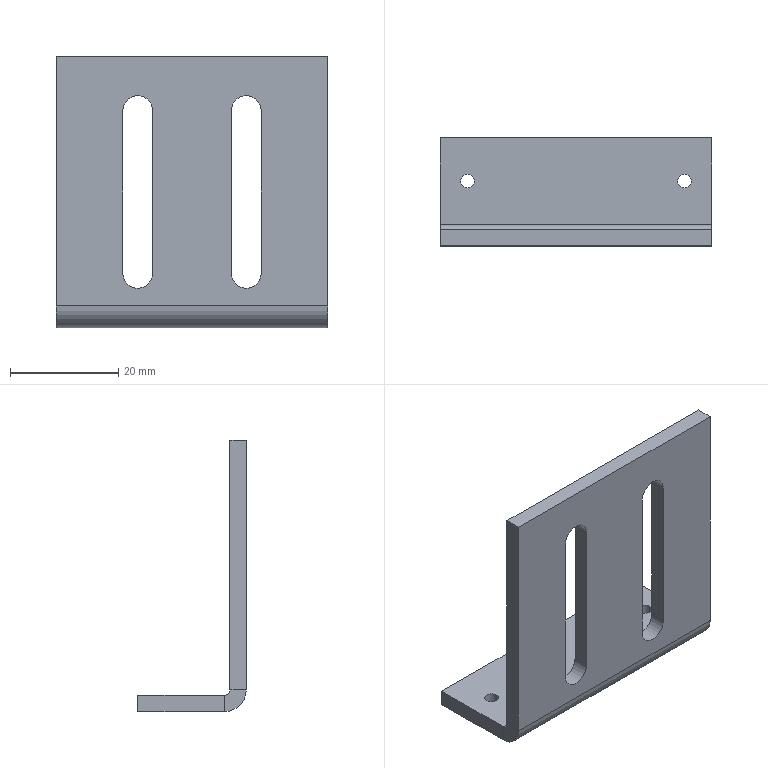Part | SolidWorks | features EdgeFlange 1, FlatPattern 1, HoleWzd 1, ICE 1, SMBaseFlange 1, SheetMetal 1 | 1 solid | 28 faces | box 50 x 20 x 50 mm | volume 8727 mm3 | plane 16 | cylinder 12 | commonest cylinder face diameters 5.5 x6 2.5 x4 2 x1 8 x1
STEP:
#1=CARTESIAN_POINT('',(18.75,2.,0.));
#2=VERTEX_POINT('',#1);
#3=CARTESIAN_POINT('',(21.25,2.,0.));
#4=VERTEX_POINT('',#3);
#5=CARTESIAN_POINT('',(20.,2.,0.));
#6=DIRECTION('',(0.,0.,1.));
#7=DIRECTION('',(1.,0.,0.));
#8=AXIS2_PLACEMENT_3D('',#5,#6,#7);
#9=CIRCLE('',#8,1.25);
#10=EDGE_CURVE('',#2,#4,#9,.T.);
#11=ORIENTED_EDGE('',*,*,#10,.T.);
#12=CARTESIAN_POINT('',(21.25,2.,-3.));
#13=VERTEX_POINT('',#12);
#14=CARTESIAN_POINT('',(21.25,2.,-3.));
#15=DIRECTION('',(0.,0.,-1.));
#16=VECTOR('',#15,1000.);
#17=LINE('',#14,#16);
#18=EDGE_CURVE('',#4,#13,#17,.T.);
#19=ORIENTED_EDGE('',*,*,#18,.T.);
#20=CARTESIAN_POINT('',(18.75,2.,-3.));
#21=VERTEX_POINT('',#20);
#22=CARTESIAN_POINT('',(20.,2.,-3.));
#23=DIRECTION('',(0.,0.,-1.));
#24=DIRECTION('',(-1.,0.,0.));
#25=AXIS2_PLACEMENT_3D('',#22,#23,#24);
#26=CIRCLE('',#25,1.25);
#27=EDGE_CURVE('',#13,#21,#26,.T.);
#28=ORIENTED_EDGE('',*,*,#27,.T.);
#29=CARTESIAN_POINT('',(18.75,2.,-3.));
#30=DIRECTION('',(0.,0.,-1.));
#31=VECTOR('',#30,1000.);
#32=LINE('',#29,#31);
#33=EDGE_CURVE('',#2,#21,#32,.T.);
#34=ORIENTED_EDGE('',*,*,#33,.F.);
#35=EDGE_LOOP('',(#11,#19,#28,#34));
#36=FACE_OUTER_BOUND('',#35,.T.);
#37=CARTESIAN_POINT('',(20.,2.,-3.));
#38=DIRECTION('',(0.,0.,-1.));
#39=DIRECTION('',(-1.,0.,0.));
#40=AXIS2_PLACEMENT_3D('',#37,#38,#39);
#41=CYLINDRICAL_SURFACE('',#40,1.25);
#42=ADVANCED_FACE('',(#36),#41,.F.);
#43=CARTESIAN_POINT('',(-21.25,2.,0.));
#44=VERTEX_POINT('',#43);
#45=CARTESIAN_POINT('',(-18.75,2.,0.));
#46=VERTEX_POINT('',#45);
#47=CARTESIAN_POINT('',(-20.,2.,0.));
#48=DIRECTION('',(0.,0.,1.));
#49=DIRECTION('',(1.,0.,0.));
#50=AXIS2_PLACEMENT_3D('',#47,#48,#49);
#51=CIRCLE('',#50,1.25);
#52=EDGE_CURVE('',#44,#46,#51,.T.);
#53=ORIENTED_EDGE('',*,*,#52,.T.);
#54=CARTESIAN_POINT('',(-18.75,2.,-3.));
#55=VERTEX_POINT('',#54);
#56=CARTESIAN_POINT('',(-18.75,2.,-3.));
#57=DIRECTION('',(0.,0.,-1.));
#58=VECTOR('',#57,1000.);
#59=LINE('',#56,#58);
#60=EDGE_CURVE('',#46,#55,#59,.T.);
#61=ORIENTED_EDGE('',*,*,#60,.T.);
#62=CARTESIAN_POINT('',(-21.25,2.,-3.));
#63=VERTEX_POINT('',#62);
#64=CARTESIAN_POINT('',(-20.,2.,-3.));
#65=DIRECTION('',(0.,0.,-1.));
#66=DIRECTION('',(-1.,0.,0.));
#67=AXIS2_PLACEMENT_3D('',#64,#65,#66);
#68=CIRCLE('',#67,1.25);
#69=EDGE_CURVE('',#55,#63,#68,.T.);
#70=ORIENTED_EDGE('',*,*,#69,.T.);
#71=CARTESIAN_POINT('',(-21.25,2.,-3.));
#72=DIRECTION('',(0.,0.,-1.));
#73=VECTOR('',#72,1000.);
#74=LINE('',#71,#73);
#75=EDGE_CURVE('',#44,#63,#74,.T.);
#76=ORIENTED_EDGE('',*,*,#75,.F.);
#77=EDGE_LOOP('',(#53,#61,#70,#76));
#78=FACE_OUTER_BOUND('',#77,.T.);
#79=CARTESIAN_POINT('',(-20.,2.,-3.));
#80=DIRECTION('',(0.,0.,-1.));
#81=DIRECTION('',(-1.,0.,0.));
#82=AXIS2_PLACEMENT_3D('',#79,#80,#81);
#83=CYLINDRICAL_SURFACE('',#82,1.25);
#84=ADVANCED_FACE('',(#78),#83,.F.);
#85=CARTESIAN_POINT('',(10.,-10.,39.75));
#86=VERTEX_POINT('',#85);
#87=CARTESIAN_POINT('',(12.75,-10.,37.));
#88=VERTEX_POINT('',#87);
#89=CARTESIAN_POINT('',(10.,-10.,37.));
#90=DIRECTION('',(0.,1.,0.));
#91=DIRECTION('',(0.,0.,1.));
#92=AXIS2_PLACEMENT_3D('',#89,#90,#91);
#93=CIRCLE('',#92,2.75);
#94=EDGE_CURVE('',#86,#88,#93,.T.);
#95=ORIENTED_EDGE('',*,*,#94,.F.);
#96=CARTESIAN_POINT('',(10.,-7.,39.75));
#97=VERTEX_POINT('',#96);
#98=CARTESIAN_POINT('',(10.,-17.,39.75));
#99=DIRECTION('',(0.,1.,0.));
#100=VECTOR('',#99,1000.);
#101=LINE('',#98,#100);
#102=EDGE_CURVE('',#86,#97,#101,.T.);
#103=ORIENTED_EDGE('',*,*,#102,.T.);
#104=CARTESIAN_POINT('',(12.75,-7.,37.));
#105=VERTEX_POINT('',#104);
#106=CARTESIAN_POINT('',(10.,-7.,37.));
#107=DIRECTION('',(0.,1.,0.));
#108=DIRECTION('',(0.,0.,1.));
#109=AXIS2_PLACEMENT_3D('',#106,#107,#108);
#110=CIRCLE('',#109,2.75);
#111=EDGE_CURVE('',#97,#105,#110,.T.);
#112=ORIENTED_EDGE('',*,*,#111,.T.);
#113=CARTESIAN_POINT('',(12.75,-17.,37.));
#114=DIRECTION('',(0.,1.,0.));
#115=VECTOR('',#114,1000.);
#116=LINE('',#113,#115);
#117=EDGE_CURVE('',#88,#105,#116,.T.);
#118=ORIENTED_EDGE('',*,*,#117,.F.);
#119=EDGE_LOOP('',(#95,#103,#112,#118));
#120=FACE_OUTER_BOUND('',#119,.T.);
#121=CARTESIAN_POINT('',(10.,-17.,37.));
#122=DIRECTION('',(0.,1.,0.));
#123=DIRECTION('',(0.,0.,1.));
#124=AXIS2_PLACEMENT_3D('',#121,#122,#123);
#125=CYLINDRICAL_SURFACE('',#124,2.75);
#126=ADVANCED_FACE('',(#120),#125,.F.);
#127=CARTESIAN_POINT('',(-10.,-10.,39.75));
#128=VERTEX_POINT('',#127);
#129=CARTESIAN_POINT('',(-7.25,-10.,37.));
#130=VERTEX_POINT('',#129);
#131=CARTESIAN_POINT('',(-10.,-10.,37.));
#132=DIRECTION('',(0.,1.,0.));
#133=DIRECTION('',(0.,0.,1.));
#134=AXIS2_PLACEMENT_3D('',#131,#132,#133);
#135=CIRCLE('',#134,2.75);
#136=EDGE_CURVE('',#128,#130,#135,.T.);
#137=ORIENTED_EDGE('',*,*,#136,.F.);
#138=CARTESIAN_POINT('',(-10.,-7.,39.75));
#139=VERTEX_POINT('',#138);
#140=CARTESIAN_POINT('',(-10.,-17.,39.75));
#141=DIRECTION('',(0.,1.,0.));
#142=VECTOR('',#141,1000.);
#143=LINE('',#140,#142);
#144=EDGE_CURVE('',#128,#139,#143,.T.);
#145=ORIENTED_EDGE('',*,*,#144,.T.);
#146=CARTESIAN_POINT('',(-7.25,-7.,37.));
#147=VERTEX_POINT('',#146);
#148=CARTESIAN_POINT('',(-10.,-7.,37.));
#149=DIRECTION('',(0.,1.,0.));
#150=DIRECTION('',(0.,0.,1.));
#151=AXIS2_PLACEMENT_3D('',#148,#149,#150);
#152=CIRCLE('',#151,2.75);
#153=EDGE_CURVE('',#139,#147,#152,.T.);
#154=ORIENTED_EDGE('',*,*,#153,.T.);
#155=CARTESIAN_POINT('',(-7.25,-17.,37.));
#156=DIRECTION('',(0.,1.,0.));
#157=VECTOR('',#156,1000.);
#158=LINE('',#155,#157);
#159=EDGE_CURVE('',#130,#147,#158,.T.);
#160=ORIENTED_EDGE('',*,*,#159,.F.);
#161=EDGE_LOOP('',(#137,#145,#154,#160));
#162=FACE_OUTER_BOUND('',#161,.T.);
#163=CARTESIAN_POINT('',(-10.,-17.,37.));
#164=DIRECTION('',(0.,1.,0.));
#165=DIRECTION('',(0.,0.,1.));
#166=AXIS2_PLACEMENT_3D('',#163,#164,#165);
#167=CYLINDRICAL_SURFACE('',#166,2.75);
#168=ADVANCED_FACE('',(#162),#167,.F.);
#169=CARTESIAN_POINT('',(25.,-6.,0.));
#170=VERTEX_POINT('',#169);
#171=CARTESIAN_POINT('',(25.,10.,0.));
#172=VERTEX_POINT('',#171);
#173=CARTESIAN_POINT('',(25.,10.,0.));
#174=DIRECTION('',(0.,1.,0.));
#175=VECTOR('',#174,1000.);
#176=LINE('',#173,#175);
#177=EDGE_CURVE('',#170,#172,#176,.T.);
#178=ORIENTED_EDGE('',*,*,#177,.F.);
#179=CARTESIAN_POINT('',(25.,-6.,-3.));
#180=VERTEX_POINT('',#179);
#181=CARTESIAN_POINT('',(25.,-6.,0.));
#182=DIRECTION('',(0.,0.,-1.));
#183=VECTOR('',#182,1000.);
#184=LINE('',#181,#183);
#185=EDGE_CURVE('',#170,#180,#184,.T.);
#186=ORIENTED_EDGE('',*,*,#185,.T.);
#187=CARTESIAN_POINT('',(25.,10.,-3.));
#188=VERTEX_POINT('',#187);
#189=CARTESIAN_POINT('',(25.,10.,-3.));
#190=DIRECTION('',(0.,1.,0.));
#191=VECTOR('',#190,1000.);
#192=LINE('',#189,#191);
#193=EDGE_CURVE('',#180,#188,#192,.T.);
#194=ORIENTED_EDGE('',*,*,#193,.T.);
#195=CARTESIAN_POINT('',(25.,10.,-3.));
#196=DIRECTION('',(0.,0.,1.));
#197=VECTOR('',#196,1000.);
#198=LINE('',#195,#197);
#199=EDGE_CURVE('',#188,#172,#198,.T.);
#200=ORIENTED_EDGE('',*,*,#199,.T.);
#201=EDGE_LOOP('',(#178,#186,#194,#200));
#202=FACE_OUTER_BOUND('',#201,.T.);
#203=CARTESIAN_POINT('',(25.,10.,-3.));
#204=DIRECTION('',(1.,0.,0.));
#205=DIRECTION('',(0.,1.,0.));
#206=AXIS2_PLACEMENT_3D('',#203,#204,#205);
#207=PLANE('',#206);
#208=ADVANCED_FACE('',(#202),#207,.T.);
#209=CARTESIAN_POINT('',(20.,2.,-3.));
#210=DIRECTION('',(0.,0.,-1.));
#211=DIRECTION('',(-1.,0.,0.));
#212=AXIS2_PLACEMENT_3D('',#209,#210,#211);
#213=CIRCLE('',#212,1.25);
#214=EDGE_CURVE('',#21,#13,#213,.T.);
#215=ORIENTED_EDGE('',*,*,#214,.F.);
#216=ORIENTED_EDGE('',*,*,#27,.F.);
#217=EDGE_LOOP('',(#215,#216));
#218=FACE_BOUND('',#217,.T.);
#219=CARTESIAN_POINT('',(-20.,2.,-3.));
#220=DIRECTION('',(0.,0.,-1.));
#221=DIRECTION('',(-1.,0.,0.));
#222=AXIS2_PLACEMENT_3D('',#219,#220,#221);
#223=CIRCLE('',#222,1.25);
#224=EDGE_CURVE('',#63,#55,#223,.T.);
#225=ORIENTED_EDGE('',*,*,#224,.F.);
#226=ORIENTED_EDGE('',*,*,#69,.F.);
#227=EDGE_LOOP('',(#225,#226));
#228=FACE_BOUND('',#227,.T.);
#229=CARTESIAN_POINT('',(-25.,-6.,-3.));
#230=VERTEX_POINT('',#229);
#231=CARTESIAN_POINT('',(25.,-6.,-3.));
#232=DIRECTION('',(-1.,0.,0.));
#233=VECTOR('',#232,1000.);
#234=LINE('',#231,#233);
#235=EDGE_CURVE('',#180,#230,#234,.T.);
#236=ORIENTED_EDGE('',*,*,#235,.T.);
#237=CARTESIAN_POINT('',(-25.,10.,-3.));
#238=VERTEX_POINT('',#237);
#239=CARTESIAN_POINT('',(-25.,10.,-3.));
#240=DIRECTION('',(0.,-1.,0.));
#241=VECTOR('',#240,1000.);
#242=LINE('',#239,#241);
#243=EDGE_CURVE('',#238,#230,#242,.T.);
#244=ORIENTED_EDGE('',*,*,#243,.F.);
#245=CARTESIAN_POINT('',(-25.,10.,-3.));
#246=DIRECTION('',(-1.,0.,0.));
#247=VECTOR('',#246,1000.);
#248=LINE('',#245,#247);
#249=EDGE_CURVE('',#188,#238,#248,.T.);
#250=ORIENTED_EDGE('',*,*,#249,.F.);
#251=ORIENTED_EDGE('',*,*,#193,.F.);
#252=EDGE_LOOP('',(#236,#244,#250,#251));
#253=FACE_OUTER_BOUND('',#252,.T.);
#254=CARTESIAN_POINT('',(0.,0.,-3.));
#255=DIRECTION('',(0.,0.,1.));
#256=DIRECTION('',(1.,0.,0.));
#257=AXIS2_PLACEMENT_3D('',#254,#255,#256);
#258=PLANE('',#257);
#259=ADVANCED_FACE('',(#218,#228,#253),#258,.F.);
#260=ORIENTED_EDGE('',*,*,#10,.F.);
#261=CARTESIAN_POINT('',(20.,2.,0.));
#262=DIRECTION('',(0.,0.,1.));
#263=DIRECTION('',(1.,0.,0.));
#264=AXIS2_PLACEMENT_3D('',#261,#262,#263);
#265=CIRCLE('',#264,1.25);
#266=EDGE_CURVE('',#4,#2,#265,.T.);
#267=ORIENTED_EDGE('',*,*,#266,.F.);
#268=EDGE_LOOP('',(#260,#267));
#269=FACE_BOUND('',#268,.T.);
#270=ORIENTED_EDGE('',*,*,#52,.F.);
#271=CARTESIAN_POINT('',(-20.,2.,0.));
#272=DIRECTION('',(0.,0.,1.));
#273=DIRECTION('',(1.,0.,0.));
#274=AXIS2_PLACEMENT_3D('',#271,#272,#273);
#275=CIRCLE('',#274,1.25);
#276=EDGE_CURVE('',#46,#44,#275,.T.);
#277=ORIENTED_EDGE('',*,*,#276,.F.);
#278=EDGE_LOOP('',(#270,#277));
#279=FACE_BOUND('',#278,.T.);
#280=CARTESIAN_POINT('',(-25.,10.,0.));
#281=VERTEX_POINT('',#280);
#282=CARTESIAN_POINT('',(-25.,-6.,0.));
#283=VERTEX_POINT('',#282);
#284=CARTESIAN_POINT('',(-25.,10.,0.));
#285=DIRECTION('',(0.,-1.,0.));
#286=VECTOR('',#285,1000.);
#287=LINE('',#284,#286);
#288=EDGE_CURVE('',#281,#283,#287,.T.);
#289=ORIENTED_EDGE('',*,*,#288,.T.);
#290=CARTESIAN_POINT('',(25.,-6.,0.));
#291=DIRECTION('',(-1.,0.,0.));
#292=VECTOR('',#291,1000.);
#293=LINE('',#290,#292);
#294=EDGE_CURVE('',#170,#283,#293,.T.);
#295=ORIENTED_EDGE('',*,*,#294,.F.);
#296=ORIENTED_EDGE('',*,*,#177,.T.);
#297=CARTESIAN_POINT('',(-25.,10.,0.));
#298=DIRECTION('',(-1.,0.,0.));
#299=VECTOR('',#298,1000.);
#300=LINE('',#297,#299);
#301=EDGE_CURVE('',#172,#281,#300,.T.);
#302=ORIENTED_EDGE('',*,*,#301,.T.);
#303=EDGE_LOOP('',(#289,#295,#296,#302));
#304=FACE_OUTER_BOUND('',#303,.T.);
#305=CARTESIAN_POINT('',(0.,0.,0.));
#306=DIRECTION('',(0.,0.,1.));
#307=DIRECTION('',(1.,0.,0.));
#308=AXIS2_PLACEMENT_3D('',#305,#306,#307);
#309=PLANE('',#308);
#310=ADVANCED_FACE('',(#269,#279,#304),#309,.T.);
#311=CARTESIAN_POINT('',(-25.,-6.,0.));
#312=DIRECTION('',(0.,0.,-1.));
#313=VECTOR('',#312,1000.);
#314=LINE('',#311,#313);
#315=EDGE_CURVE('',#283,#230,#314,.T.);
#316=ORIENTED_EDGE('',*,*,#315,.F.);
#317=ORIENTED_EDGE('',*,*,#288,.F.);
#318=CARTESIAN_POINT('',(-25.,10.,-3.));
#319=DIRECTION('',(0.,0.,1.));
#320=VECTOR('',#319,1000.);
#321=LINE('',#318,#320);
#322=EDGE_CURVE('',#238,#281,#321,.T.);
#323=ORIENTED_EDGE('',*,*,#322,.F.);
#324=ORIENTED_EDGE('',*,*,#243,.T.);
#325=EDGE_LOOP('',(#316,#317,#323,#324));
#326=FACE_OUTER_BOUND('',#325,.T.);
#327=CARTESIAN_POINT('',(-25.,10.,-3.));
#328=DIRECTION('',(-1.,0.,0.));
#329=DIRECTION('',(0.,-1.,0.));
#330=AXIS2_PLACEMENT_3D('',#327,#328,#329);
#331=PLANE('',#330);
#332=ADVANCED_FACE('',(#326),#331,.T.);
#333=ORIENTED_EDGE('',*,*,#301,.F.);
#334=ORIENTED_EDGE('',*,*,#199,.F.);
#335=ORIENTED_EDGE('',*,*,#249,.T.);
#336=ORIENTED_EDGE('',*,*,#322,.T.);
#337=EDGE_LOOP('',(#333,#334,#335,#336));
#338=FACE_OUTER_BOUND('',#337,.T.);
#339=CARTESIAN_POINT('',(-25.,10.,-3.));
#340=DIRECTION('',(0.,1.,0.));
#341=DIRECTION('',(0.,0.,1.));
#342=AXIS2_PLACEMENT_3D('',#339,#340,#341);
#343=PLANE('',#342);
#344=ADVANCED_FACE('',(#338),#343,.T.);
#345=CARTESIAN_POINT('',(-25.,-7.,1.));
#346=VERTEX_POINT('',#345);
#347=CARTESIAN_POINT('',(-25.,-10.,1.));
#348=VERTEX_POINT('',#347);
#349=CARTESIAN_POINT('',(-25.,-10.,1.));
#350=DIRECTION('',(0.,-1.,0.));
#351=VECTOR('',#350,1000.);
#352=LINE('',#349,#351);
#353=EDGE_CURVE('',#346,#348,#352,.T.);
#354=ORIENTED_EDGE('',*,*,#353,.F.);
#355=CARTESIAN_POINT('',(-25.,-6.,1.));
#356=DIRECTION('',(-1.,0.,0.));
#357=DIRECTION('',(0.,0.,-1.));
#358=AXIS2_PLACEMENT_3D('',#355,#356,#357);
#359=CIRCLE('',#358,1.);
#360=EDGE_CURVE('',#283,#346,#359,.T.);
#361=ORIENTED_EDGE('',*,*,#360,.F.);
#362=ORIENTED_EDGE('',*,*,#315,.T.);
#363=CARTESIAN_POINT('',(-25.,-6.,1.));
#364=DIRECTION('',(-1.,0.,0.));
#365=DIRECTION('',(0.,0.,-1.));
#366=AXIS2_PLACEMENT_3D('',#363,#364,#365);
#367=CIRCLE('',#366,4.);
#368=EDGE_CURVE('',#230,#348,#367,.T.);
#369=ORIENTED_EDGE('',*,*,#368,.T.);
#370=EDGE_LOOP('',(#354,#361,#362,#369));
#371=FACE_OUTER_BOUND('',#370,.T.);
#372=CARTESIAN_POINT('',(-25.,-6.,1.));
#373=DIRECTION('',(-1.,0.,0.));
#374=DIRECTION('',(0.,0.,1.));
#375=AXIS2_PLACEMENT_3D('',#372,#373,#374);
#376=PLANE('',#375);
#377=ADVANCED_FACE('',(#371),#376,.T.);
#378=CARTESIAN_POINT('',(25.,-7.,1.));
#379=VERTEX_POINT('',#378);
#380=CARTESIAN_POINT('',(25.,-6.,1.));
#381=DIRECTION('',(1.,0.,0.));
#382=DIRECTION('',(0.,0.,-1.));
#383=AXIS2_PLACEMENT_3D('',#380,#381,#382);
#384=CIRCLE('',#383,1.);
#385=EDGE_CURVE('',#379,#170,#384,.T.);
#386=ORIENTED_EDGE('',*,*,#385,.F.);
#387=CARTESIAN_POINT('',(25.,-10.,1.));
#388=VERTEX_POINT('',#387);
#389=CARTESIAN_POINT('',(25.,-7.,1.));
#390=DIRECTION('',(0.,-1.,0.));
#391=VECTOR('',#390,1000.);
#392=LINE('',#389,#391);
#393=EDGE_CURVE('',#379,#388,#392,.T.);
#394=ORIENTED_EDGE('',*,*,#393,.T.);
#395=CARTESIAN_POINT('',(25.,-6.,1.));
#396=DIRECTION('',(1.,0.,0.));
#397=DIRECTION('',(0.,0.,-1.));
#398=AXIS2_PLACEMENT_3D('',#395,#396,#397);
#399=CIRCLE('',#398,4.);
#400=EDGE_CURVE('',#388,#180,#399,.T.);
#401=ORIENTED_EDGE('',*,*,#400,.T.);
#402=ORIENTED_EDGE('',*,*,#185,.F.);
#403=EDGE_LOOP('',(#386,#394,#401,#402));
#404=FACE_OUTER_BOUND('',#403,.T.);
#405=CARTESIAN_POINT('',(25.,-6.,1.));
#406=DIRECTION('',(-1.,0.,0.));
#407=DIRECTION('',(0.,0.,1.));
#408=AXIS2_PLACEMENT_3D('',#405,#406,#407);
#409=PLANE('',#408);
#410=ADVANCED_FACE('',(#404),#409,.F.);
#411=ORIENTED_EDGE('',*,*,#235,.F.);
#412=ORIENTED_EDGE('',*,*,#400,.F.);
#413=CARTESIAN_POINT('',(-25.,-10.,1.));
#414=DIRECTION('',(-1.,0.,0.));
#415=VECTOR('',#414,1000.);
#416=LINE('',#413,#415);
#417=EDGE_CURVE('',#388,#348,#416,.T.);
#418=ORIENTED_EDGE('',*,*,#417,.T.);
#419=ORIENTED_EDGE('',*,*,#368,.F.);
#420=EDGE_LOOP('',(#411,#412,#418,#419));
#421=FACE_OUTER_BOUND('',#420,.T.);
#422=CARTESIAN_POINT('',(25.,-6.,1.));
#423=DIRECTION('',(1.,0.,0.));
#424=DIRECTION('',(0.,-1.,0.));
#425=AXIS2_PLACEMENT_3D('',#422,#423,#424);
#426=CYLINDRICAL_SURFACE('',#425,4.);
#427=ADVANCED_FACE('',(#421),#426,.T.);
#428=ORIENTED_EDGE('',*,*,#294,.T.);
#429=ORIENTED_EDGE('',*,*,#360,.T.);
#430=CARTESIAN_POINT('',(-25.,-7.,1.));
#431=DIRECTION('',(1.,0.,0.));
#432=VECTOR('',#431,1000.);
#433=LINE('',#430,#432);
#434=EDGE_CURVE('',#346,#379,#433,.T.);
#435=ORIENTED_EDGE('',*,*,#434,.T.);
#436=ORIENTED_EDGE('',*,*,#385,.T.);
#437=EDGE_LOOP('',(#428,#429,#435,#436));
#438=FACE_OUTER_BOUND('',#437,.T.);
#439=CARTESIAN_POINT('',(25.,-6.,1.));
#440=DIRECTION('',(1.,0.,0.));
#441=DIRECTION('',(0.,-1.,0.));
#442=AXIS2_PLACEMENT_3D('',#439,#440,#441);
#443=CYLINDRICAL_SURFACE('',#442,1.);
#444=ADVANCED_FACE('',(#438),#443,.F.);
#445=ORIENTED_EDGE('',*,*,#353,.T.);
#446=CARTESIAN_POINT('',(-25.,-10.,47.));
#447=VERTEX_POINT('',#446);
#448=CARTESIAN_POINT('',(-25.,-10.,0.));
#449=DIRECTION('',(0.,0.,-1.));
#450=VECTOR('',#449,1000.);
#451=LINE('',#448,#450);
#452=EDGE_CURVE('',#447,#348,#451,.T.);
#453=ORIENTED_EDGE('',*,*,#452,.F.);
#454=CARTESIAN_POINT('',(-25.,-7.,47.));
#455=VERTEX_POINT('',#454);
#456=CARTESIAN_POINT('',(-25.,-10.,47.));
#457=DIRECTION('',(0.,1.,0.));
#458=VECTOR('',#457,1000.);
#459=LINE('',#456,#458);
#460=EDGE_CURVE('',#447,#455,#459,.T.);
#461=ORIENTED_EDGE('',*,*,#460,.T.);
#462=CARTESIAN_POINT('',(-25.,-7.,0.));
#463=DIRECTION('',(0.,0.,-1.));
#464=VECTOR('',#463,1000.);
#465=LINE('',#462,#464);
#466=EDGE_CURVE('',#455,#346,#465,.T.);
#467=ORIENTED_EDGE('',*,*,#466,.T.);
#468=EDGE_LOOP('',(#445,#453,#461,#467));
#469=FACE_OUTER_BOUND('',#468,.T.);
#470=CARTESIAN_POINT('',(-25.,-10.,0.));
#471=DIRECTION('',(1.,0.,0.));
#472=DIRECTION('',(0.,0.,-1.));
#473=AXIS2_PLACEMENT_3D('',#470,#471,#472);
#474=PLANE('',#473);
#475=ADVANCED_FACE('',(#469),#474,.F.);
#476=ORIENTED_EDGE('',*,*,#393,.F.);
#477=CARTESIAN_POINT('',(25.,-7.,47.));
#478=VERTEX_POINT('',#477);
#479=CARTESIAN_POINT('',(25.,-7.,47.));
#480=DIRECTION('',(0.,0.,1.));
#481=VECTOR('',#480,1000.);
#482=LINE('',#479,#481);
#483=EDGE_CURVE('',#379,#478,#482,.T.);
#484=ORIENTED_EDGE('',*,*,#483,.T.);
#485=CARTESIAN_POINT('',(25.,-10.,47.));
#486=VERTEX_POINT('',#485);
#487=CARTESIAN_POINT('',(25.,-10.,47.));
#488=DIRECTION('',(0.,1.,0.));
#489=VECTOR('',#488,1000.);
#490=LINE('',#487,#489);
#491=EDGE_CURVE('',#486,#478,#490,.T.);
#492=ORIENTED_EDGE('',*,*,#491,.F.);
#493=CARTESIAN_POINT('',(25.,-10.,0.));
#494=DIRECTION('',(0.,0.,1.));
#495=VECTOR('',#494,1000.);
#496=LINE('',#493,#495);
#497=EDGE_CURVE('',#388,#486,#496,.T.);
#498=ORIENTED_EDGE('',*,*,#497,.F.);
#499=EDGE_LOOP('',(#476,#484,#492,#498));
#500=FACE_OUTER_BOUND('',#499,.T.);
#501=CARTESIAN_POINT('',(25.,-10.,47.));
#502=DIRECTION('',(-1.,0.,0.));
#503=DIRECTION('',(0.,0.,1.));
#504=AXIS2_PLACEMENT_3D('',#501,#502,#503);
#505=PLANE('',#504);
#506=ADVANCED_FACE('',(#500),#505,.F.);
#507=CARTESIAN_POINT('',(12.75,-10.,7.));
#508=VERTEX_POINT('',#507);
#509=CARTESIAN_POINT('',(7.25,-10.,7.));
#510=VERTEX_POINT('',#509);
#511=CARTESIAN_POINT('',(10.,-10.,7.));
#512=DIRECTION('',(0.,1.,0.));
#513=DIRECTION('',(0.,0.,1.));
#514=AXIS2_PLACEMENT_3D('',#511,#512,#513);
#515=CIRCLE('',#514,2.75);
#516=EDGE_CURVE('',#508,#510,#515,.T.);
#517=ORIENTED_EDGE('',*,*,#516,.T.);
#518=CARTESIAN_POINT('',(7.25,-10.,37.));
#519=VERTEX_POINT('',#518);
#520=CARTESIAN_POINT('',(7.25,-10.,0.));
#521=DIRECTION('',(0.,0.,1.));
#522=VECTOR('',#521,1000.);
#523=LINE('',#520,#522);
#524=EDGE_CURVE('',#510,#519,#523,.T.);
#525=ORIENTED_EDGE('',*,*,#524,.T.);
#526=CARTESIAN_POINT('',(10.,-10.,37.));
#527=DIRECTION('',(0.,1.,0.));
#528=DIRECTION('',(0.,0.,1.));
#529=AXIS2_PLACEMENT_3D('',#526,#527,#528);
#530=CIRCLE('',#529,2.75);
#531=EDGE_CURVE('',#519,#86,#530,.T.);
#532=ORIENTED_EDGE('',*,*,#531,.T.);
#533=ORIENTED_EDGE('',*,*,#94,.T.);
#534=CARTESIAN_POINT('',(12.75,-10.,0.));
#535=DIRECTION('',(0.,0.,1.));
#536=VECTOR('',#535,1000.);
#537=LINE('',#534,#536);
#538=EDGE_CURVE('',#508,#88,#537,.T.);
#539=ORIENTED_EDGE('',*,*,#538,.F.);
#540=EDGE_LOOP('',(#517,#525,#532,#533,#539));
#541=FACE_BOUND('',#540,.T.);
#542=CARTESIAN_POINT('',(-7.25,-10.,7.));
#543=VERTEX_POINT('',#542);
#544=CARTESIAN_POINT('',(-7.25,-10.,0.));
#545=DIRECTION('',(0.,0.,1.));
#546=VECTOR('',#545,1000.);
#547=LINE('',#544,#546);
#548=EDGE_CURVE('',#543,#130,#547,.T.);
#549=ORIENTED_EDGE('',*,*,#548,.F.);
#550=CARTESIAN_POINT('',(-12.75,-10.,7.));
#551=VERTEX_POINT('',#550);
#552=CARTESIAN_POINT('',(-10.,-10.,7.));
#553=DIRECTION('',(0.,1.,0.));
#554=DIRECTION('',(0.,0.,1.));
#555=AXIS2_PLACEMENT_3D('',#552,#553,#554);
#556=CIRCLE('',#555,2.75);
#557=EDGE_CURVE('',#543,#551,#556,.T.);
#558=ORIENTED_EDGE('',*,*,#557,.T.);
#559=CARTESIAN_POINT('',(-12.75,-10.,37.));
#560=VERTEX_POINT('',#559);
#561=CARTESIAN_POINT('',(-12.75,-10.,0.));
#562=DIRECTION('',(0.,0.,1.));
#563=VECTOR('',#562,1000.);
#564=LINE('',#561,#563);
#565=EDGE_CURVE('',#551,#560,#564,.T.);
#566=ORIENTED_EDGE('',*,*,#565,.T.);
#567=CARTESIAN_POINT('',(-10.,-10.,37.));
#568=DIRECTION('',(0.,1.,0.));
#569=DIRECTION('',(0.,0.,1.));
#570=AXIS2_PLACEMENT_3D('',#567,#568,#569);
#571=CIRCLE('',#570,2.75);
#572=EDGE_CURVE('',#560,#128,#571,.T.);
#573=ORIENTED_EDGE('',*,*,#572,.T.);
#574=ORIENTED_EDGE('',*,*,#136,.T.);
#575=EDGE_LOOP('',(#549,#558,#566,#573,#574));
#576=FACE_BOUND('',#575,.T.);
#577=ORIENTED_EDGE('',*,*,#417,.F.);
#578=ORIENTED_EDGE('',*,*,#497,.T.);
#579=CARTESIAN_POINT('',(0.,-10.,47.));
#580=DIRECTION('',(-1.,0.,0.));
#581=VECTOR('',#580,1000.);
#582=LINE('',#579,#581);
#583=EDGE_CURVE('',#486,#447,#582,.T.);
#584=ORIENTED_EDGE('',*,*,#583,.T.);
#585=ORIENTED_EDGE('',*,*,#452,.T.);
#586=EDGE_LOOP('',(#577,#578,#584,#585));
#587=FACE_OUTER_BOUND('',#586,.T.);
#588=CARTESIAN_POINT('',(0.,-10.,0.));
#589=DIRECTION('',(0.,1.,0.));
#590=DIRECTION('',(0.,0.,1.));
#591=AXIS2_PLACEMENT_3D('',#588,#589,#590);
#592=PLANE('',#591);
#593=ADVANCED_FACE('',(#541,#576,#587),#592,.F.);
#594=CARTESIAN_POINT('',(7.25,-7.,7.));
#595=VERTEX_POINT('',#594);
#596=CARTESIAN_POINT('',(7.25,-7.,37.));
#597=VERTEX_POINT('',#596);
#598=CARTESIAN_POINT('',(7.25,-7.,7.));
#599=DIRECTION('',(0.,0.,1.));
#600=VECTOR('',#599,1000.);
#601=LINE('',#598,#600);
#602=EDGE_CURVE('',#595,#597,#601,.T.);
#603=ORIENTED_EDGE('',*,*,#602,.F.);
#604=CARTESIAN_POINT('',(12.75,-7.,7.));
#605=VERTEX_POINT('',#604);
#606=CARTESIAN_POINT('',(10.,-7.,7.));
#607=DIRECTION('',(0.,1.,0.));
#608=DIRECTION('',(0.,0.,1.));
#609=AXIS2_PLACEMENT_3D('',#606,#607,#608);
#610=CIRCLE('',#609,2.75);
#611=EDGE_CURVE('',#605,#595,#610,.T.);
#612=ORIENTED_EDGE('',*,*,#611,.F.);
#613=CARTESIAN_POINT('',(12.75,-7.,7.));
#614=DIRECTION('',(0.,0.,1.));
#615=VECTOR('',#614,1000.);
#616=LINE('',#613,#615);
#617=EDGE_CURVE('',#605,#105,#616,.T.);
#618=ORIENTED_EDGE('',*,*,#617,.T.);
#619=ORIENTED_EDGE('',*,*,#111,.F.);
#620=CARTESIAN_POINT('',(10.,-7.,37.));
#621=DIRECTION('',(0.,1.,0.));
#622=DIRECTION('',(0.,0.,1.));
#623=AXIS2_PLACEMENT_3D('',#620,#621,#622);
#624=CIRCLE('',#623,2.75);
#625=EDGE_CURVE('',#597,#97,#624,.T.);
#626=ORIENTED_EDGE('',*,*,#625,.F.);
#627=EDGE_LOOP('',(#603,#612,#618,#619,#626));
#628=FACE_BOUND('',#627,.T.);
#629=CARTESIAN_POINT('',(-7.25,-7.,7.));
#630=VERTEX_POINT('',#629);
#631=CARTESIAN_POINT('',(-12.75,-7.,7.));
#632=VERTEX_POINT('',#631);
#633=CARTESIAN_POINT('',(-10.,-7.,7.));
#634=DIRECTION('',(0.,1.,0.));
#635=DIRECTION('',(0.,0.,1.));
#636=AXIS2_PLACEMENT_3D('',#633,#634,#635);
#637=CIRCLE('',#636,2.75);
#638=EDGE_CURVE('',#630,#632,#637,.T.);
#639=ORIENTED_EDGE('',*,*,#638,.F.);
#640=CARTESIAN_POINT('',(-7.25,-7.,7.));
#641=DIRECTION('',(0.,0.,1.));
#642=VECTOR('',#641,1000.);
#643=LINE('',#640,#642);
#644=EDGE_CURVE('',#630,#147,#643,.T.);
#645=ORIENTED_EDGE('',*,*,#644,.T.);
#646=ORIENTED_EDGE('',*,*,#153,.F.);
#647=CARTESIAN_POINT('',(-12.75,-7.,37.));
#648=VERTEX_POINT('',#647);
#649=CARTESIAN_POINT('',(-10.,-7.,37.));
#650=DIRECTION('',(0.,1.,0.));
#651=DIRECTION('',(0.,0.,1.));
#652=AXIS2_PLACEMENT_3D('',#649,#650,#651);
#653=CIRCLE('',#652,2.75);
#654=EDGE_CURVE('',#648,#139,#653,.T.);
#655=ORIENTED_EDGE('',*,*,#654,.F.);
#656=CARTESIAN_POINT('',(-12.75,-7.,7.));
#657=DIRECTION('',(0.,0.,1.));
#658=VECTOR('',#657,1000.);
#659=LINE('',#656,#658);
#660=EDGE_CURVE('',#632,#648,#659,.T.);
#661=ORIENTED_EDGE('',*,*,#660,.F.);
#662=EDGE_LOOP('',(#639,#645,#646,#655,#661));
#663=FACE_BOUND('',#662,.T.);
#664=ORIENTED_EDGE('',*,*,#483,.F.);
#665=ORIENTED_EDGE('',*,*,#434,.F.);
#666=ORIENTED_EDGE('',*,*,#466,.F.);
#667=CARTESIAN_POINT('',(-25.,-7.,47.));
#668=DIRECTION('',(-1.,0.,0.));
#669=VECTOR('',#668,1000.);
#670=LINE('',#667,#669);
#671=EDGE_CURVE('',#478,#455,#670,.T.);
#672=ORIENTED_EDGE('',*,*,#671,.F.);
#673=EDGE_LOOP('',(#664,#665,#666,#672));
#674=FACE_OUTER_BOUND('',#673,.T.);
#675=CARTESIAN_POINT('',(0.,-7.,0.));
#676=DIRECTION('',(0.,1.,0.));
#677=DIRECTION('',(0.,0.,1.));
#678=AXIS2_PLACEMENT_3D('',#675,#676,#677);
#679=PLANE('',#678);
#680=ADVANCED_FACE('',(#628,#663,#674),#679,.T.);
#681=ORIENTED_EDGE('',*,*,#671,.T.);
#682=ORIENTED_EDGE('',*,*,#460,.F.);
#683=ORIENTED_EDGE('',*,*,#583,.F.);
#684=ORIENTED_EDGE('',*,*,#491,.T.);
#685=EDGE_LOOP('',(#681,#682,#683,#684));
#686=FACE_OUTER_BOUND('',#685,.T.);
#687=CARTESIAN_POINT('',(-25.,-10.,47.));
#688=DIRECTION('',(0.,0.,-1.));
#689=DIRECTION('',(0.,1.,0.));
#690=AXIS2_PLACEMENT_3D('',#687,#688,#689);
#691=PLANE('',#690);
#692=ADVANCED_FACE('',(#686),#691,.F.);
#693=CARTESIAN_POINT('',(-7.25,-17.,7.));
#694=DIRECTION('',(0.,1.,0.));
#695=VECTOR('',#694,1000.);
#696=LINE('',#693,#695);
#697=EDGE_CURVE('',#543,#630,#696,.T.);
#698=ORIENTED_EDGE('',*,*,#697,.T.);
#699=ORIENTED_EDGE('',*,*,#638,.T.);
#700=CARTESIAN_POINT('',(-12.75,-17.,7.));
#701=DIRECTION('',(0.,1.,0.));
#702=VECTOR('',#701,1000.);
#703=LINE('',#700,#702);
#704=EDGE_CURVE('',#551,#632,#703,.T.);
#705=ORIENTED_EDGE('',*,*,#704,.F.);
#706=ORIENTED_EDGE('',*,*,#557,.F.);
#707=EDGE_LOOP('',(#698,#699,#705,#706));
#708=FACE_OUTER_BOUND('',#707,.T.);
#709=CARTESIAN_POINT('',(-10.,-17.,7.));
#710=DIRECTION('',(0.,1.,0.));
#711=DIRECTION('',(0.,0.,1.));
#712=AXIS2_PLACEMENT_3D('',#709,#710,#711);
#713=CYLINDRICAL_SURFACE('',#712,2.75);
#714=ADVANCED_FACE('',(#708),#713,.F.);
#715=ORIENTED_EDGE('',*,*,#548,.T.);
#716=ORIENTED_EDGE('',*,*,#159,.T.);
#717=ORIENTED_EDGE('',*,*,#644,.F.);
#718=ORIENTED_EDGE('',*,*,#697,.F.);
#719=EDGE_LOOP('',(#715,#716,#717,#718));
#720=FACE_OUTER_BOUND('',#719,.T.);
#721=CARTESIAN_POINT('',(-7.25,-17.,7.));
#722=DIRECTION('',(-1.,0.,0.));
#723=DIRECTION('',(0.,0.,1.));
#724=AXIS2_PLACEMENT_3D('',#721,#722,#723);
#725=PLANE('',#724);
#726=ADVANCED_FACE('',(#720),#725,.T.);
#727=ORIENTED_EDGE('',*,*,#144,.F.);
#728=ORIENTED_EDGE('',*,*,#572,.F.);
#729=CARTESIAN_POINT('',(-12.75,-17.,37.));
#730=DIRECTION('',(0.,1.,0.));
#731=VECTOR('',#730,1000.);
#732=LINE('',#729,#731);
#733=EDGE_CURVE('',#560,#648,#732,.T.);
#734=ORIENTED_EDGE('',*,*,#733,.T.);
#735=ORIENTED_EDGE('',*,*,#654,.T.);
#736=EDGE_LOOP('',(#727,#728,#734,#735));
#737=FACE_OUTER_BOUND('',#736,.T.);
#738=CARTESIAN_POINT('',(-10.,-17.,37.));
#739=DIRECTION('',(0.,1.,0.));
#740=DIRECTION('',(0.,0.,1.));
#741=AXIS2_PLACEMENT_3D('',#738,#739,#740);
#742=CYLINDRICAL_SURFACE('',#741,2.75);
#743=ADVANCED_FACE('',(#737),#742,.F.);
#744=ORIENTED_EDGE('',*,*,#704,.T.);
#745=ORIENTED_EDGE('',*,*,#660,.T.);
#746=ORIENTED_EDGE('',*,*,#733,.F.);
#747=ORIENTED_EDGE('',*,*,#565,.F.);
#748=EDGE_LOOP('',(#744,#745,#746,#747));
#749=FACE_OUTER_BOUND('',#748,.T.);
#750=CARTESIAN_POINT('',(-12.75,-17.,7.));
#751=DIRECTION('',(-1.,0.,0.));
#752=DIRECTION('',(0.,0.,1.));
#753=AXIS2_PLACEMENT_3D('',#750,#751,#752);
#754=PLANE('',#753);
#755=ADVANCED_FACE('',(#749),#754,.F.);
#756=CARTESIAN_POINT('',(7.25,-17.,7.));
#757=DIRECTION('',(0.,1.,0.));
#758=VECTOR('',#757,1000.);
#759=LINE('',#756,#758);
#760=EDGE_CURVE('',#510,#595,#759,.T.);
#761=ORIENTED_EDGE('',*,*,#760,.T.);
#762=ORIENTED_EDGE('',*,*,#602,.T.);
#763=CARTESIAN_POINT('',(7.25,-17.,37.));
#764=DIRECTION('',(0.,1.,0.));
#765=VECTOR('',#764,1000.);
#766=LINE('',#763,#765);
#767=EDGE_CURVE('',#519,#597,#766,.T.);
#768=ORIENTED_EDGE('',*,*,#767,.F.);
#769=ORIENTED_EDGE('',*,*,#524,.F.);
#770=EDGE_LOOP('',(#761,#762,#768,#769));
#771=FACE_OUTER_BOUND('',#770,.T.);
#772=CARTESIAN_POINT('',(7.25,-17.,7.));
#773=DIRECTION('',(-1.,0.,0.));
#774=DIRECTION('',(0.,0.,1.));
#775=AXIS2_PLACEMENT_3D('',#772,#773,#774);
#776=PLANE('',#775);
#777=ADVANCED_FACE('',(#771),#776,.F.);
#778=CARTESIAN_POINT('',(12.75,-17.,7.));
#779=DIRECTION('',(0.,1.,0.));
#780=VECTOR('',#779,1000.);
#781=LINE('',#778,#780);
#782=EDGE_CURVE('',#508,#605,#781,.T.);
#783=ORIENTED_EDGE('',*,*,#782,.T.);
#784=ORIENTED_EDGE('',*,*,#611,.T.);
#785=ORIENTED_EDGE('',*,*,#760,.F.);
#786=ORIENTED_EDGE('',*,*,#516,.F.);
#787=EDGE_LOOP('',(#783,#784,#785,#786));
#788=FACE_OUTER_BOUND('',#787,.T.);
#789=CARTESIAN_POINT('',(10.,-17.,7.));
#790=DIRECTION('',(0.,1.,0.));
#791=DIRECTION('',(0.,0.,1.));
#792=AXIS2_PLACEMENT_3D('',#789,#790,#791);
#793=CYLINDRICAL_SURFACE('',#792,2.75);
#794=ADVANCED_FACE('',(#788),#793,.F.);
#795=ORIENTED_EDGE('',*,*,#538,.T.);
#796=ORIENTED_EDGE('',*,*,#117,.T.);
#797=ORIENTED_EDGE('',*,*,#617,.F.);
#798=ORIENTED_EDGE('',*,*,#782,.F.);
#799=EDGE_LOOP('',(#795,#796,#797,#798));
#800=FACE_OUTER_BOUND('',#799,.T.);
#801=CARTESIAN_POINT('',(12.75,-17.,7.));
#802=DIRECTION('',(-1.,0.,0.));
#803=DIRECTION('',(0.,0.,1.));
#804=AXIS2_PLACEMENT_3D('',#801,#802,#803);
#805=PLANE('',#804);
#806=ADVANCED_FACE('',(#800),#805,.T.);
#807=ORIENTED_EDGE('',*,*,#102,.F.);
#808=ORIENTED_EDGE('',*,*,#531,.F.);
#809=ORIENTED_EDGE('',*,*,#767,.T.);
#810=ORIENTED_EDGE('',*,*,#625,.T.);
#811=EDGE_LOOP('',(#807,#808,#809,#810));
#812=FACE_OUTER_BOUND('',#811,.T.);
#813=CARTESIAN_POINT('',(10.,-17.,37.));
#814=DIRECTION('',(0.,1.,0.));
#815=DIRECTION('',(0.,0.,1.));
#816=AXIS2_PLACEMENT_3D('',#813,#814,#815);
#817=CYLINDRICAL_SURFACE('',#816,2.75);
#818=ADVANCED_FACE('',(#812),#817,.F.);
#819=ORIENTED_EDGE('',*,*,#60,.F.);
#820=ORIENTED_EDGE('',*,*,#276,.T.);
#821=ORIENTED_EDGE('',*,*,#75,.T.);
#822=ORIENTED_EDGE('',*,*,#224,.T.);
#823=EDGE_LOOP('',(#819,#820,#821,#822));
#824=FACE_OUTER_BOUND('',#823,.T.);
#825=CARTESIAN_POINT('',(-20.,2.,-3.));
#826=DIRECTION('',(0.,0.,-1.));
#827=DIRECTION('',(-1.,0.,0.));
#828=AXIS2_PLACEMENT_3D('',#825,#826,#827);
#829=CYLINDRICAL_SURFACE('',#828,1.25);
#830=ADVANCED_FACE('',(#824),#829,.F.);
#831=ORIENTED_EDGE('',*,*,#18,.F.);
#832=ORIENTED_EDGE('',*,*,#266,.T.);
#833=ORIENTED_EDGE('',*,*,#33,.T.);
#834=ORIENTED_EDGE('',*,*,#214,.T.);
#835=EDGE_LOOP('',(#831,#832,#833,#834));
#836=FACE_OUTER_BOUND('',#835,.T.);
#837=CARTESIAN_POINT('',(20.,2.,-3.));
#838=DIRECTION('',(0.,0.,-1.));
#839=DIRECTION('',(-1.,0.,0.));
#840=AXIS2_PLACEMENT_3D('',#837,#838,#839);
#841=CYLINDRICAL_SURFACE('',#840,1.25);
#842=ADVANCED_FACE('',(#836),#841,.F.);
#843=CLOSED_SHELL('',(#42,#84,#126,#168,#208,#259,#310,#332,#344,#377,#410,#427,#444,#475,#506,#593,#680,#692,#714,#726,#743,#755,#777,#794,#806,#818,#830,#842));
#844=MANIFOLD_SOLID_BREP('',#843);
#845=CARTESIAN_POINT('',(0.,0.,0.));
#846=DIRECTION('',(0.,0.,1.));
#847=DIRECTION('',(1.,0.,0.));
#848=AXIS2_PLACEMENT_3D('',#845,#846,#847);
#849=(LENGTH_UNIT()NAMED_UNIT(*)SI_UNIT(.MILLI.,.METRE.));
#850=UNCERTAINTY_MEASURE_WITH_UNIT(LENGTH_MEASURE(0.00001),#849,'','');
#851=(NAMED_UNIT(*)PLANE_ANGLE_UNIT()SI_UNIT($,.RADIAN.));
#852=(NAMED_UNIT(*)SI_UNIT($,.STERADIAN.)SOLID_ANGLE_UNIT());
#853=(GEOMETRIC_REPRESENTATION_CONTEXT(3)GLOBAL_UNCERTAINTY_ASSIGNED_CONTEXT((#850))GLOBAL_UNIT_ASSIGNED_CONTEXT((#849,#851,#852))REPRESENTATION_CONTEXT('',''));
#854=ADVANCED_BREP_SHAPE_REPRESENTATION('',(#844,#848),#853);